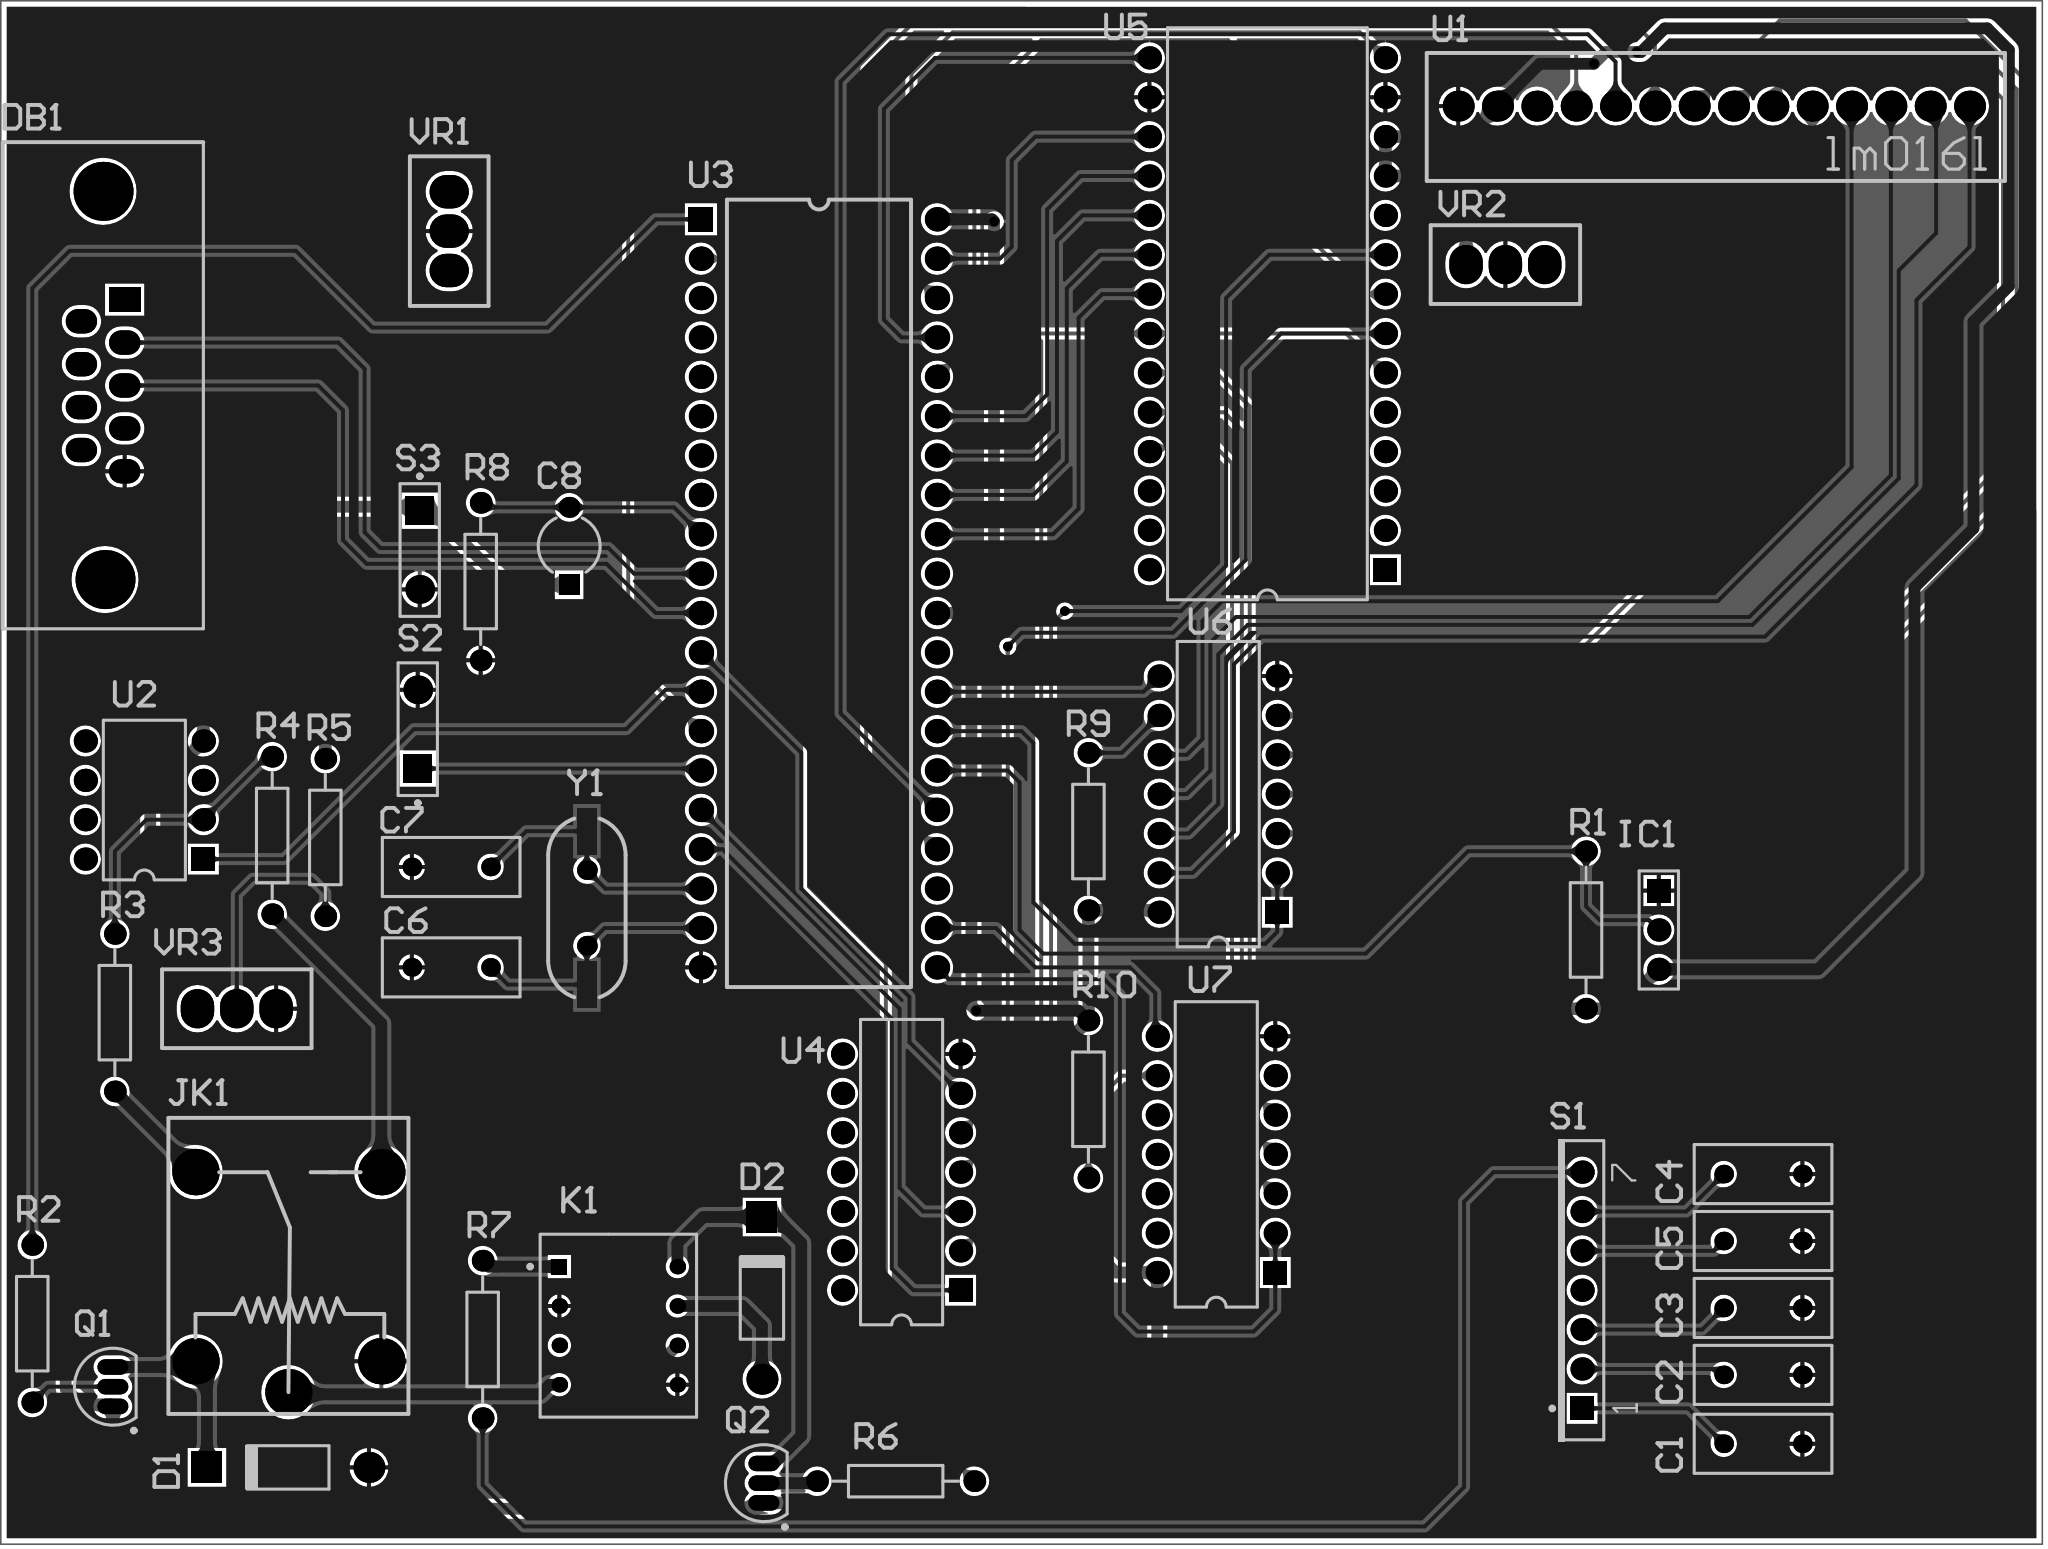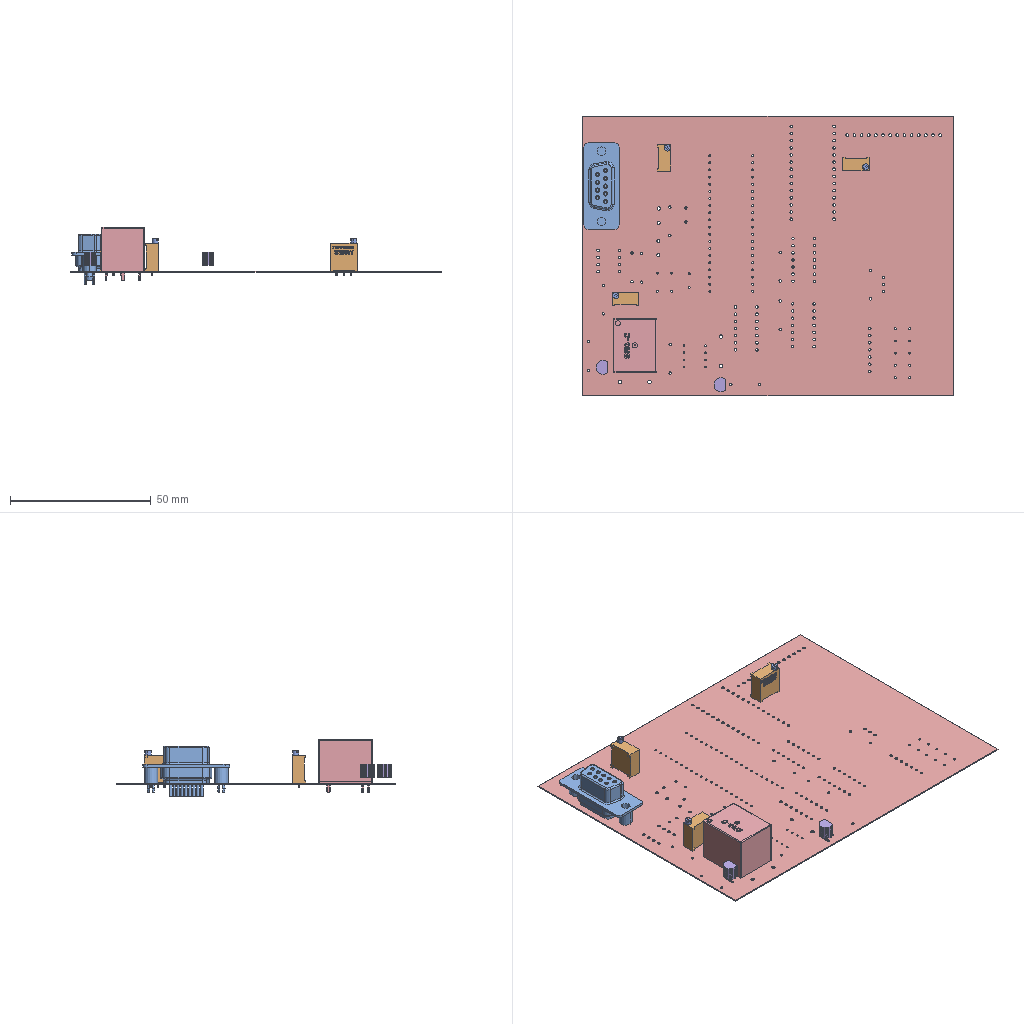Circuit board layout | Altium Designer | box 131.8 x 99.6 x 20.3 mm
Layer stack:
# Altium Designer layer stack of  (unit mm; dielectric type: 0 none, 1 core, 2 prepreg, 3 surface material)
index,name,kind,layer,copper_thickness_mm,dielectric_type,dielectric_thickness_mm,dielectric_material,dielectric_constant
0,Top Paste,other,,,,,,
1,Top Overlay,other,,,,,,
2,Top Solder,dielectric,,,3,0.0102,Solder Resist,3.5
3,Top Layer,copper,Top Layer,0.0356,,,,
4,Dielectric 1,dielectric,,,0,0.32,FR-4,4.8
5,Bottom Layer,copper,Bottom Layer,0.0356,,,,
6,Bottom Solder,dielectric,,,3,0.0102,Solder Resist,3.5
7,Bottom Overlay,other,,,,,,
8,Bottom Paste,other,,,,,,
# drill layer pairs: low layer,high layer
drill_pair,Top Layer,Bottom Layer
Part placement:
Designator,Comment,Layer,Footprint,Center-X(mm),Center-Y(mm),Rotation
Y1,12M,TopLayer,XTAL_US,90.297,68.353,270
VR3,4.7K,TopLayer,3296W,67.691,61.849,180
VR2,RESVR,TopLayer,3296W,149.606,109.855,360
VR1,RESVR,TopLayer,3296W,81.407,112.014,90
U7,SN74LS164N,TopLayer,646-06,130.937,52.451,90
U6,SN74LS164N,TopLayer,646-06,131.064,75.692,90
U5,ADC0808N,TopLayer,N028,134.239,106.68,90
U4,SN74LS04N,TopLayer,646-06,110.617,51.308,90
U3,AT89C51,TopLayer,DIP40,105.283,88.646,0
U2,MAX942MJA,TopLayer,JA8,61.722,75.311,90
U1,LM016L,TopLayer,LM016L,163.068,120.079,360
S3,SW-PB,TopLayer,SPST-2,79.502,91.44,270
S2,SW-PB,TopLayer,SPST-2,79.375,79.883,90
S1,SW-6WAY,TopLayer,SW-7,154.559,43.688,90
R10,10K,TopLayer,AXIAL-0.4,122.682,56.007,90
R9,10K,TopLayer,AXIAL-0.4,122.682,73.279,270
R8,10K,TopLayer,AXIAL-0.4,83.439,89.408,90
R7,100,TopLayer,AXIAL-0.4,83.566,40.513,90
R6,100,TopLayer,AXIAL-0.4,110.236,31.369,360
R5,1K,TopLayer,AXIAL-0.4,73.406,72.898,270
R4,10K,TopLayer,AXIAL-0.4,69.977,73.025,270
R3,10M,TopLayer,AXIAL-0.4,59.817,61.595,270
R2,100,TopLayer,AXIAL-0.4,54.483,41.529,90
R1,4.7K,TopLayer,AXIAL-0.4,154.813,66.929,270
Q2,2N3906,TopLayer,TO-92A,101.727,31.242,0
Q1,2N3906,TopLayer,TO-92A,59.69,37.465,0
K1,G2R-24-DC5,TopLayer,DIP-P8,92.329,41.402,270
JK1,W172DIP-1,TopLayer,SRD-C_BK,71.024,44.208,90
IC1,DS18B20,TopLayer,HDR1X3,159.512,66.929,270
DB1,DB9/F,TopLayer,DB9/F/180,59.055,102.057,90
D2,Diode 1N4001,TopLayer,DO-41,101.6,43.18,90
D1,Diode 1N4001,TopLayer,DO-41,70.993,32.258,180
C8,10UF,TopLayer,CAPR5-4X5,89.154,91.694,90
C7,30PF,TopLayer,RAD-0.2,81.534,70.993,360
C6,30PF,TopLayer,RAD-0.2,81.534,64.516,360
C5,342UF,TopLayer,RAD-0.2,166.243,46.863,180
C4,67UF,TopLayer,RAD-0.2,166.243,51.181,180
C3,700NF,TopLayer,RAD-0.2,166.243,42.545,180
C2,200NF,TopLayer,RAD-0.2,166.243,38.227,180
C1,20NF,TopLayer,RAD-0.2,166.243,33.782,180
Pad and via stacks:
# Altium Designer via and pad stacks of  (unit mm). Each distinct definition once, with the count of objects using it.
# via: kind,start_layer,end_layer,hole_mm,diameter_mm,mode(0 simple;1 top-mid-bottom;2 full stack),diameter_per_layer,count,example_net
# pad: kind,layer,hole_mm,hole_type(0 round;1 square;2 slot),plating,top_size,top_shape(1 round;2 rect;3 octagon;9 rounded rect),mid_size,bottom_size,mode,footprint,size_per_layer,count,example
pad,Multi-Layer,0.9,0,plated,1.5x1.5,2,1.5x1.5,1.5x1.5,0,HDR1X3,,1,IC1.1
pad,Multi-Layer,0.9,0,plated,1.5x1.5,1,1.5x1.5,1.5x1.5,0,HDR1X3,,2,IC1.2
pad,Multi-Layer,0.7112,0,plated,1.575x1.575,2,1.575x1.575,1.575x1.575,0,DIP40,,1,U3.1
pad,Multi-Layer,0.7112,0,plated,1.575x1.575,1,1.575x1.575,1.575x1.575,0,DIP40,,39,U3.2
pad,Multi-Layer,0.7,0,plated,1.2x1.2,1,1.2x1.2,1.2x1.2,0,RAD-0.2,,14,C6.2
pad,Multi-Layer,0.7112,0,plated,1.27x1.27,1,1.27x1.27,1.27x1.27,0,XTAL_US,,2,Y1.2
pad,Multi-Layer,0.9652,0,plated,1.575x2.032,2,1.575x2.032,1.575x2.032,0,DB9/F/180,,1,DB1.1
pad,Multi-Layer,0.9652,0,plated,1.575x2.032,1,1.575x2.032,1.575x2.032,0,DB9/F/180,,8,DB1.2
pad,Multi-Layer,2.794,0,plated,3.81x3.81,1,3.81x3.81,3.81x3.81,0,DB9/F/180,,2,DB1.0
pad,Multi-Layer,0.9,0,plated,1.5x1.5,1,1.5x1.5,1.5x1.5,0,646-06,,39,U4.8
pad,Multi-Layer,0.9,0,plated,1.5x1.5,2,1.5x1.5,1.5x1.5,0,646-06,,3,U4.1
pad,Multi-Layer,0.8,0,plated,1.35x1.35,1,1.35x1.35,1.35x1.35,0,CAPR5-4X5,,1,C8.2
pad,Multi-Layer,0.8,0,plated,1.35x1.35,2,1.35x1.35,1.35x1.35,0,CAPR5-4X5,,1,C8.1
pad,Multi-Layer,0.85,0,plated,1.4x1.4,1,1.4x1.4,1.4x1.4,0,AXIAL-0.4,,20,R8.1
pad,Multi-Layer,1.1,0,plated,1.85x1.85,2,1.85x1.85,1.85x1.85,0,SPST-2,,2,S3.1
pad,Multi-Layer,1.1,0,plated,1.85x1.85,1,1.85x1.85,1.85x1.85,0,SPST-2,,2,S3.2
pad,Multi-Layer,0.9,0,plated,1.5x1.5,1,1.5x1.5,1.5x1.5,0,N028,,27,U5.15
pad,Multi-Layer,0.9,0,plated,1.5x1.5,2,1.5x1.5,1.5x1.5,0,N028,,1,U5.1
pad,Multi-Layer,1,2,plated,2x2,1,2x2,2x2,0,LM016L,,14,U1.4
pad,Multi-Layer,0.889,0,plated,2.159x2.54,1,2.159x2.54,2.159x2.54,0,3296W,,9,VR1.3
pad,Multi-Layer,0.9,0,plated,1.5x1.5,1,1.5x1.5,1.5x1.5,0,SW-7,,6,S1.7
pad,Multi-Layer,0.9,0,plated,1.5x1.5,2,1.5x1.5,1.5x1.5,0,SW-7,,1,S1.1
pad,Multi-Layer,0.9,0,plated,2x1,1,2x1,2x1,0,TO-92A,,6,Q1.3
pad,Multi-Layer,0.9,0,plated,1.5x1.5,2,1.5x1.5,1.5x1.5,0,JA8,,1,U2.1
pad,Multi-Layer,0.9,0,plated,1.5x1.5,1,1.5x1.5,1.5x1.5,0,JA8,,7,U2.2
pad,Multi-Layer,1.6,0,plated,3x3,1,3x3,3x3,0,SRD-C_BK,,5,JK1.3
pad,Multi-Layer,1.2,0,plated,2x2,1,2x2,2x2,0,DO-41,,2,D1.1
pad,Multi-Layer,1.2,0,plated,2x2,2,2x2,2x2,0,DO-41,,2,D1.2
pad,Multi-Layer,0.6,0,plated,1x1,1,1x1,1x1,0,DIP-P8,,7,K1.8
pad,Multi-Layer,0.6,0,plated,1x1,2,1x1,1x1,0,DIP-P8,,1,K1.1
pad,Top Layer,0,0,plated,3x1.27,2,3x1.27,3x1.27,0,XTAL_US,,2,Y1.2
via,Top Layer,Bottom Layer,0.3048,0.6096,0,,6,VCC
Copper pours:
name,layer,net,type(0 solid;1 hatched;2 none)
D,Top Layer,GND,0
D,Bottom Layer,GND,0
Design rules, without the lines most boards share:
# Altium Designer design rules of  (exported by Altium Designer, unit mm)
# columns: name | kind | enabled | priority | scope1 | scope2 | descriptor | typed fields (field=value)
SilkToSilkClearance | 55 | enabled | 1 | All | All | Silk to Silk (Clearance=0mil) (All),(All) |
SilkToSolderMaskClearance | 54 | enabled | 1 | IsPad | All | Silk To Solder Mask (Clearance=0mil) (IsPad),(All) |
MinimumSolderMaskSliver | 53 | enabled | 1 | All | All | Minimum Solder Mask Sliver (Gap=0mil) (All),(All) |
HoleToHoleClearance | 52 | enabled | 1 | All | All | Hole To Hole Clearance (Gap=10mil) (All),(All) | gap=0.254
DiffPairsRouting | 51 | enabled | 1 | All | All | Differential Pairs Uncoupled Length using the Gap Constraints (Min=10mil) (Max=10mil) (Prefered=10mil)  and Width Constraints (Min=15mil) (Max=15mil) (Prefered=15mil) (All) |
SolderMaskExpansion | 13 | enabled | 1 | All | All | Solder Mask Expansion (Expansion =4mil) (All) | expansion=0.1016
PasteMaskExpansion | 14 | enabled | 1 | All | All | Paste Mask Expansion (Expansion =0mil) (All) | expansion=0
RoutingVias | 11 | enabled | 1 | All | All | Routing Via (MinHoleWidth=28mil) (MaxHoleWidth=28mil) (PreferredHoleWidth=28mil) (MinWidth=50mil) (MaxWidth=50mil) (PreferedWidth=50mil) (All) | via_min_hole=0.7112 via_max_hole=0.7112 via_preferred_diameter=1.27 via_preferred_hole=0.7112
Width | 2 | enabled | 1 | All | All | Width Constraint (Min=10mil) (Max=30mil) (Preferred=10mil) (All) |
PolygonConnect | 20 | enabled | 1 | All | All | Polygon Connect Rule(Relief Connect )(Conductor Width=10mil) (Relief Angle=90 Angle) (Entries=4) (Air Gap Width=10mil) (All),(All) | connect_style(0=relief,1=direct,2=none)=0 relief_conductor_width=0.254 relief_entries=4
PlaneConnect | 6 | enabled | 1 | All | All | Power Plane Connect Rule(Relief Connect )(Expansion=20mil) (Conductor Width=10mil) (Air Gap=10mil) (Entries=4) (All) | relief_conductor_width=0.254 relief_entries=4 relief_expansion=0.508
Clearance | 0 | enabled | 1 | All | All | Clearance Constraint (Gap=10mil) (All),(All) | gap=0.254
Classes set for this board:
# Altium Designer classes of  (member kind: 0 net, 1 component, 2 from-to, 3 pad, 4 layer, 5 differential pair, 6 design channel, 7 polygon, 8 structure, 9 xSignal)
# columns: class name | member kind | superclass | members
Sheet2 | 1 | no | C6; C7; C8; DB1; R8; R9; R10; S3; U3; U4; U5; U6; U7; Y1;
Sheet1 | 1 | no | C1; C2; C3; C4; C5; D1; D2; IC1; JK1; K1; Q1; Q2; R1; R2; R3; R4; R5; R6; R7; S1; S2; U1; U2; VR1; VR2; VR3;